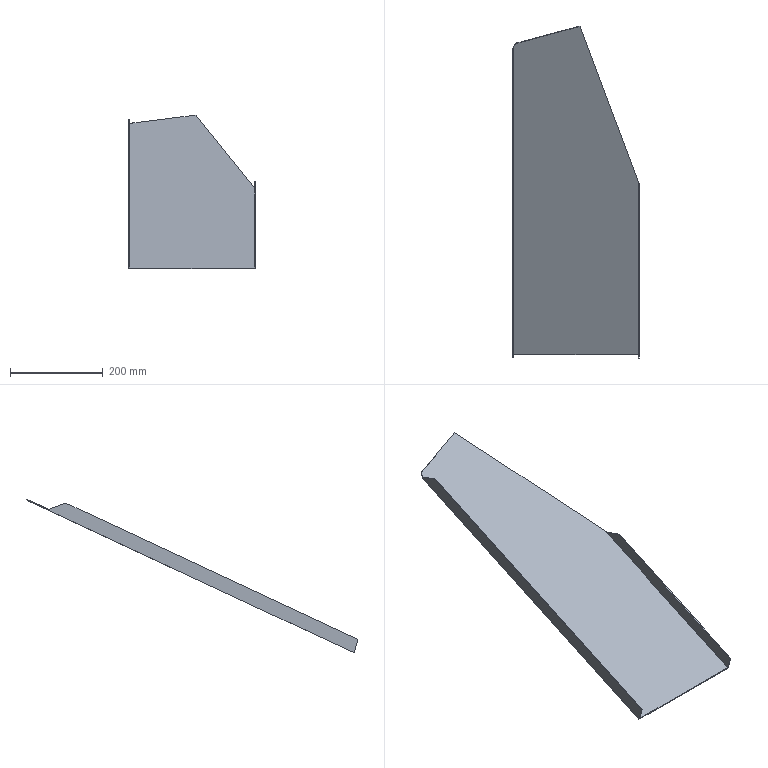Part | NX | features solid 2 | 1 solid | 14 faces | box 271.348 x 713.846 x 331.008 mm | volume 430827 mm3 | plane 13 | spline 1
STEP:
#1=CARTESIAN_POINT('',(380.079,-710.47,-537.234));
#2=VERTEX_POINT('',#1);
#3=CARTESIAN_POINT('',(112.731,-710.47,-537.234));
#4=VERTEX_POINT('',#3);
#5=CARTESIAN_POINT('',(177.1,-710.47,-537.234));
#6=DIRECTION('',(-1.,0.,0.));
#7=VECTOR('',#6,1000.);
#8=LINE('',#5,#7);
#9=EDGE_CURVE('',#2,#4,#8,.T.);
#10=ORIENTED_EDGE('',*,*,#9,.F.);
#11=CARTESIAN_POINT('',(380.079,-342.448,-365.622));
#12=VERTEX_POINT('',#11);
#13=CARTESIAN_POINT('',(380.079,-25.721,-217.93));
#14=DIRECTION('',(0.,0.9063,0.4226));
#15=VECTOR('',#14,1000.);
#16=LINE('',#13,#15);
#17=EDGE_CURVE('',#2,#12,#16,.T.);
#18=ORIENTED_EDGE('',*,*,#17,.T.);
#19=CARTESIAN_POINT('',(382.079,-342.448,-365.622));
#20=VERTEX_POINT('',#19);
#21=CARTESIAN_POINT('',(382.079,-342.448,-365.622));
#22=DIRECTION('',(-1.,0.,0.));
#23=VECTOR('',#22,1000.);
#24=LINE('',#21,#23);
#25=EDGE_CURVE('',#12,#20,#24,.F.);
#26=ORIENTED_EDGE('',*,*,#25,.T.);
#27=CARTESIAN_POINT('',(255.072,-4.828,-208.187));
#28=VERTEX_POINT('',#27);
#29=CARTESIAN_POINT('',(255.072,-4.828,-208.187));
#30=DIRECTION('',(0.3227,-0.8578,-0.4));
#31=VECTOR('',#30,1000.);
#32=LINE('',#29,#31);
#33=EDGE_CURVE('',#28,#20,#32,.T.);
#34=ORIENTED_EDGE('',*,*,#33,.F.);
#35=CARTESIAN_POINT('',(244.53,-7.653,-209.505));
#36=VERTEX_POINT('',#35);
#37=CARTESIAN_POINT('',(255.072,-4.828,-208.187));
#38=CARTESIAN_POINT('',(251.558,-5.77,-208.626));
#39=CARTESIAN_POINT('',(248.044,-6.711,-209.066));
#40=CARTESIAN_POINT('',(244.53,-7.653,-209.505));
#41=B_SPLINE_CURVE_WITH_KNOTS('',3,(#37,#38,#39,#40),.UNSPECIFIED.,.F.,.F.,(4,4),(0.,1.),.PIECEWISE_BEZIER_KNOTS.);
#42=EDGE_CURVE('',#28,#36,#41,.T.);
#43=ORIENTED_EDGE('',*,*,#42,.T.);
#44=CARTESIAN_POINT('',(110.731,-52.513,-230.423));
#45=VERTEX_POINT('',#44);
#46=CARTESIAN_POINT('',(105.417,-66.15,-236.782));
#47=CARTESIAN_POINT('',(107.811,-60.006,-233.917));
#48=CARTESIAN_POINT('',(110.205,-53.862,-231.052));
#49=CARTESIAN_POINT('',(112.599,-47.718,-228.187));
#50=CARTESIAN_POINT('',(112.723,-47.398,-228.038));
#51=CARTESIAN_POINT('',(112.863,-47.087,-227.893));
#52=CARTESIAN_POINT('',(113.169,-46.477,-227.609));
#53=CARTESIAN_POINT('',(113.336,-46.18,-227.47));
#54=CARTESIAN_POINT('',(113.695,-45.599,-227.199));
#55=CARTESIAN_POINT('',(113.888,-45.315,-227.067));
#56=CARTESIAN_POINT('',(114.298,-44.762,-226.809));
#57=CARTESIAN_POINT('',(114.517,-44.493,-226.683));
#58=CARTESIAN_POINT('',(114.865,-44.1,-226.5));
#59=CARTESIAN_POINT('',(114.985,-43.97,-226.44));
#60=CARTESIAN_POINT('',(115.169,-43.779,-226.351));
#61=CARTESIAN_POINT('',(115.232,-43.716,-226.321));
#62=CARTESIAN_POINT('',(115.358,-43.591,-226.263));
#63=CARTESIAN_POINT('',(115.422,-43.53,-226.234));
#64=CARTESIAN_POINT('',(115.745,-43.225,-226.092));
#65=CARTESIAN_POINT('',(116.014,-42.994,-225.984));
#66=CARTESIAN_POINT('',(116.436,-42.666,-225.831));
#67=CARTESIAN_POINT('',(116.579,-42.56,-225.782));
#68=CARTESIAN_POINT('',(116.873,-42.355,-225.686));
#69=CARTESIAN_POINT('',(117.023,-42.256,-225.64));
#70=CARTESIAN_POINT('',(117.33,-42.066,-225.551));
#71=CARTESIAN_POINT('',(117.487,-41.974,-225.509));
#72=CARTESIAN_POINT('',(117.688,-41.865,-225.458));
#73=CARTESIAN_POINT('',(117.729,-41.844,-225.448));
#74=CARTESIAN_POINT('',(117.81,-41.801,-225.428));
#75=CARTESIAN_POINT('',(117.932,-41.739,-225.399));
#76=CARTESIAN_POINT('',(118.055,-41.679,-225.371));
#77=CARTESIAN_POINT('',(118.303,-41.564,-225.318));
#78=CARTESIAN_POINT('',(118.471,-41.493,-225.285));
#79=CARTESIAN_POINT('',(118.809,-41.363,-225.224));
#80=CARTESIAN_POINT('',(118.981,-41.304,-225.196));
#81=CARTESIAN_POINT('',(119.198,-41.238,-225.166));
#82=CARTESIAN_POINT('',(119.263,-41.219,-225.157));
#83=CARTESIAN_POINT('',(119.329,-41.201,-225.148));
#84=CARTESIAN_POINT('',(119.372,-41.189,-225.143));
#85=CARTESIAN_POINT('',(119.394,-41.183,-225.14));
#86=CARTESIAN_POINT('',(119.504,-41.154,-225.126));
#87=CARTESIAN_POINT('',(119.767,-41.083,-225.093));
#88=CARTESIAN_POINT('',(120.733,-40.824,-224.973));
#89=CARTESIAN_POINT('',(123.016,-40.213,-224.687));
#90=CARTESIAN_POINT('',(130.742,-38.142,-223.722));
#91=CARTESIAN_POINT('',(149.005,-33.249,-221.44));
#92=CARTESIAN_POINT('',(188.339,-22.709,-216.526));
#93=CARTESIAN_POINT('',(222.053,-13.676,-212.313));
#94=CARTESIAN_POINT('',(244.53,-7.653,-209.505));
#95=CARTESIAN_POINT('',(251.273,-5.846,-208.662));
#96=CARTESIAN_POINT('',(258.016,-4.039,-207.82));
#97=CARTESIAN_POINT('',(264.759,-2.233,-206.977));
#98=B_SPLINE_CURVE_WITH_KNOTS('',3,(#46,#47,#48,#49,#50,#51,#52,#53,#54,#55,#56,#57,#58,#59,#60,#61,#62,#63,#64,#65,#66,#67,#68,#69,#70,#71,#72,#73,#74,#75,#76,#77,#78,#79,#80,#81,#82,#83,#84,#85,#86,#87,#88,#89,#90,#91,#92,#93,#94,#95,#96,#97),.UNSPECIFIED.,.F.,.F.,(4,3,2,2,2,2,2,2,2,2,2,2,2,2,1,2,2,2,1,2,2,1,1,1,1,1,1,3,4),(-0.15,0.,0.007812,0.01562,0.02344,0.03125,0.03516,0.03711,0.03906,0.04687,0.05078,0.05469,0.05859,0.05957,0.06055,0.0625,0.06641,0.07031,0.07129,0.07178,0.07227,0.07422,0.07812,0.09375,0.125,0.25,0.5,1.,1.15),.UNSPECIFIED.);
#99=EDGE_CURVE('',#45,#36,#98,.T.);
#100=ORIENTED_EDGE('',*,*,#99,.F.);
#101=CARTESIAN_POINT('',(112.731,-52.513,-230.423));
#102=VERTEX_POINT('',#101);
#103=CARTESIAN_POINT('',(110.731,-52.513,-230.423));
#104=DIRECTION('',(-1.,0.,0.));
#105=VECTOR('',#104,1000.);
#106=LINE('',#103,#105);
#107=EDGE_CURVE('',#45,#102,#106,.F.);
#108=ORIENTED_EDGE('',*,*,#107,.T.);
#109=CARTESIAN_POINT('',(112.731,-25.721,-217.93));
#110=DIRECTION('',(0.,-0.9063,-0.4226));
#111=VECTOR('',#110,1000.);
#112=LINE('',#109,#111);
#113=EDGE_CURVE('',#102,#4,#112,.T.);
#114=ORIENTED_EDGE('',*,*,#113,.T.);
#115=EDGE_LOOP('',(#10,#18,#26,#34,#43,#100,#108,#114));
#116=FACE_BOUND('',#115,.T.);
#117=CARTESIAN_POINT('',(177.1,-25.721,-217.93));
#118=DIRECTION('',(0.,-0.4226,0.9063));
#119=DIRECTION('',(0.,-0.9063,-0.4226));
#120=AXIS2_PLACEMENT_3D('',#117,#118,#119);
#121=PLANE('',#120);
#122=ADVANCED_FACE('',(#116),#121,.T.);
#123=CARTESIAN_POINT('',(110.731,-51.668,-232.236));
#124=VERTEX_POINT('',#123);
#125=CARTESIAN_POINT('',(244.53,-6.808,-211.317));
#126=VERTEX_POINT('',#125);
#127=CARTESIAN_POINT('',(105.417,-65.305,-238.595));
#128=CARTESIAN_POINT('',(107.811,-59.161,-235.73));
#129=CARTESIAN_POINT('',(110.205,-53.017,-232.865));
#130=CARTESIAN_POINT('',(112.599,-46.873,-230.));
#131=CARTESIAN_POINT('',(112.723,-46.553,-229.851));
#132=CARTESIAN_POINT('',(112.863,-46.241,-229.705));
#133=CARTESIAN_POINT('',(113.169,-45.632,-229.421));
#134=CARTESIAN_POINT('',(113.336,-45.335,-229.283));
#135=CARTESIAN_POINT('',(113.695,-44.754,-229.012));
#136=CARTESIAN_POINT('',(113.888,-44.47,-228.879));
#137=CARTESIAN_POINT('',(114.298,-43.917,-228.622));
#138=CARTESIAN_POINT('',(114.517,-43.648,-228.496));
#139=CARTESIAN_POINT('',(114.865,-43.254,-228.313));
#140=CARTESIAN_POINT('',(114.985,-43.125,-228.252));
#141=CARTESIAN_POINT('',(115.169,-42.934,-228.163));
#142=CARTESIAN_POINT('',(115.232,-42.871,-228.134));
#143=CARTESIAN_POINT('',(115.358,-42.746,-228.076));
#144=CARTESIAN_POINT('',(115.422,-42.685,-228.047));
#145=CARTESIAN_POINT('',(115.745,-42.38,-227.905));
#146=CARTESIAN_POINT('',(116.014,-42.148,-227.797));
#147=CARTESIAN_POINT('',(116.436,-41.821,-227.644));
#148=CARTESIAN_POINT('',(116.579,-41.715,-227.595));
#149=CARTESIAN_POINT('',(116.873,-41.51,-227.499));
#150=CARTESIAN_POINT('',(117.023,-41.411,-227.453));
#151=CARTESIAN_POINT('',(117.33,-41.22,-227.364));
#152=CARTESIAN_POINT('',(117.487,-41.129,-227.321));
#153=CARTESIAN_POINT('',(117.688,-41.02,-227.271));
#154=CARTESIAN_POINT('',(117.729,-40.999,-227.261));
#155=CARTESIAN_POINT('',(117.81,-40.956,-227.241));
#156=CARTESIAN_POINT('',(117.932,-40.894,-227.212));
#157=CARTESIAN_POINT('',(118.055,-40.834,-227.184));
#158=CARTESIAN_POINT('',(118.303,-40.719,-227.13));
#159=CARTESIAN_POINT('',(118.471,-40.648,-227.097));
#160=CARTESIAN_POINT('',(118.809,-40.518,-227.037));
#161=CARTESIAN_POINT('',(118.981,-40.459,-227.009));
#162=CARTESIAN_POINT('',(119.198,-40.393,-226.978));
#163=CARTESIAN_POINT('',(119.263,-40.374,-226.969));
#164=CARTESIAN_POINT('',(119.329,-40.356,-226.961));
#165=CARTESIAN_POINT('',(119.372,-40.344,-226.955));
#166=CARTESIAN_POINT('',(119.394,-40.338,-226.952));
#167=CARTESIAN_POINT('',(119.504,-40.308,-226.939));
#168=CARTESIAN_POINT('',(119.767,-40.238,-226.906));
#169=CARTESIAN_POINT('',(120.733,-39.979,-226.785));
#170=CARTESIAN_POINT('',(123.016,-39.367,-226.5));
#171=CARTESIAN_POINT('',(130.742,-37.297,-225.535));
#172=CARTESIAN_POINT('',(149.005,-32.404,-223.253));
#173=CARTESIAN_POINT('',(188.339,-21.864,-218.338));
#174=CARTESIAN_POINT('',(222.053,-12.83,-214.126));
#175=CARTESIAN_POINT('',(244.53,-6.808,-211.317));
#176=CARTESIAN_POINT('',(251.273,-5.001,-210.475));
#177=CARTESIAN_POINT('',(258.016,-3.194,-209.632));
#178=CARTESIAN_POINT('',(264.759,-1.387,-208.79));
#179=B_SPLINE_CURVE_WITH_KNOTS('',3,(#127,#128,#129,#130,#131,#132,#133,#134,#135,#136,#137,#138,#139,#140,#141,#142,#143,#144,#145,#146,#147,#148,#149,#150,#151,#152,#153,#154,#155,#156,#157,#158,#159,#160,#161,#162,#163,#164,#165,#166,#167,#168,#169,#170,#171,#172,#173,#174,#175,#176,#177,#178),.UNSPECIFIED.,.F.,.F.,(4,3,2,2,2,2,2,2,2,2,2,2,2,2,1,2,2,2,1,2,2,1,1,1,1,1,1,3,4),(-0.15,0.,0.007812,0.01562,0.02344,0.03125,0.03516,0.03711,0.03906,0.04687,0.05078,0.05469,0.05859,0.05957,0.06055,0.0625,0.06641,0.07031,0.07129,0.07178,0.07227,0.07422,0.07812,0.09375,0.125,0.25,0.5,1.,1.15),.UNSPECIFIED.);
#180=EDGE_CURVE('',#124,#126,#179,.T.);
#181=ORIENTED_EDGE('',*,*,#180,.F.);
#182=CARTESIAN_POINT('',(110.731,-52.091,-231.33));
#183=DIRECTION('',(0.,0.4226,-0.9063));
#184=VECTOR('',#183,1000.);
#185=LINE('',#182,#184);
#186=EDGE_CURVE('',#45,#124,#185,.T.);
#187=ORIENTED_EDGE('',*,*,#186,.F.);
#188=ORIENTED_EDGE('',*,*,#99,.T.);
#189=CARTESIAN_POINT('',(244.53,-7.653,-209.505));
#190=DIRECTION('',(0.,0.4226,-0.9063));
#191=VECTOR('',#190,1000.);
#192=LINE('',#189,#191);
#193=EDGE_CURVE('',#36,#126,#192,.T.);
#194=ORIENTED_EDGE('',*,*,#193,.T.);
#195=EDGE_LOOP('',(#181,#187,#188,#194));
#196=FACE_BOUND('',#195,.T.);
#197=CARTESIAN_POINT('',(110.731,-52.513,-230.423));
#198=CARTESIAN_POINT('',(110.731,-51.668,-232.236));
#199=CARTESIAN_POINT('',(111.249,-51.183,-229.803));
#200=CARTESIAN_POINT('',(111.249,-50.338,-231.616));
#201=CARTESIAN_POINT('',(112.026,-49.189,-228.873));
#202=CARTESIAN_POINT('',(112.026,-48.344,-230.686));
#203=CARTESIAN_POINT('',(113.062,-46.528,-227.632));
#204=CARTESIAN_POINT('',(113.062,-45.682,-229.445));
#205=CARTESIAN_POINT('',(114.237,-44.751,-226.804));
#206=CARTESIAN_POINT('',(114.237,-43.906,-228.616));
#207=CARTESIAN_POINT('',(115.746,-43.133,-226.049));
#208=CARTESIAN_POINT('',(115.746,-42.288,-227.862));
#209=CARTESIAN_POINT('',(117.264,-42.047,-225.543));
#210=CARTESIAN_POINT('',(117.264,-41.202,-227.355));
#211=CARTESIAN_POINT('',(118.643,-41.392,-225.237));
#212=CARTESIAN_POINT('',(118.643,-40.547,-227.05));
#213=CARTESIAN_POINT('',(120.096,-40.991,-225.05));
#214=CARTESIAN_POINT('',(120.096,-40.145,-226.863));
#215=CARTESIAN_POINT('',(122.655,-40.312,-224.734));
#216=CARTESIAN_POINT('',(122.655,-39.467,-226.547));
#217=CARTESIAN_POINT('',(126.302,-39.331,-224.276));
#218=CARTESIAN_POINT('',(126.302,-38.486,-226.089));
#219=CARTESIAN_POINT('',(132.141,-37.768,-223.548));
#220=CARTESIAN_POINT('',(132.141,-36.923,-225.36));
#221=CARTESIAN_POINT('',(139.438,-35.812,-222.635));
#222=CARTESIAN_POINT('',(139.438,-34.967,-224.448));
#223=CARTESIAN_POINT('',(148.196,-33.466,-221.541));
#224=CARTESIAN_POINT('',(148.196,-32.62,-223.354));
#225=CARTESIAN_POINT('',(156.954,-31.119,-220.447));
#226=CARTESIAN_POINT('',(156.954,-30.274,-222.26));
#227=CARTESIAN_POINT('',(165.711,-28.772,-219.353));
#228=CARTESIAN_POINT('',(165.711,-27.927,-221.165));
#229=CARTESIAN_POINT('',(177.388,-25.644,-217.894));
#230=CARTESIAN_POINT('',(177.388,-24.798,-219.706));
#231=CARTESIAN_POINT('',(203.661,-18.604,-214.611));
#232=CARTESIAN_POINT('',(203.661,-17.759,-216.424));
#233=CARTESIAN_POINT('',(227.015,-12.346,-211.693));
#234=CARTESIAN_POINT('',(227.015,-11.501,-213.506));
#235=CARTESIAN_POINT('',(244.53,-7.653,-209.505));
#236=CARTESIAN_POINT('',(244.53,-6.808,-211.317));
#237=B_SPLINE_SURFACE_WITH_KNOTS('',3,1,((#197,#198),(#199,#200),(#201,#202),(#203,#204),(#205,#206),(#207,#208),(#209,#210),(#211,#212),(#213,#214),(#215,#216),(#217,#218),(#219,#220),(#221,#222),(#223,#224),(#225,#226),(#227,#228),(#229,#230),(#231,#232),(#233,#234),(#235,#236)),.UNSPECIFIED.,.F.,.F.,.F.,(4,1,1,1,1,1,1,1,1,1,1,1,1,1,1,1,1,4),(2,2),(-0.03902,-0.006552,0.009682,0.02592,0.04215,0.05839,0.0665,0.07462,0.09086,0.1233,0.1558,0.2207,0.2857,0.3506,0.4156,0.4805,0.6104,1.),(0.,1.),.UNSPECIFIED.);
#238=ADVANCED_FACE('',(#196),#237,.T.);
#239=CARTESIAN_POINT('',(255.072,-3.983,-210.));
#240=VERTEX_POINT('',#239);
#241=CARTESIAN_POINT('',(255.072,-3.983,-210.));
#242=CARTESIAN_POINT('',(251.558,-4.925,-210.439));
#243=CARTESIAN_POINT('',(248.044,-5.866,-210.878));
#244=CARTESIAN_POINT('',(244.53,-6.808,-211.317));
#245=B_SPLINE_CURVE_WITH_KNOTS('',3,(#241,#242,#243,#244),.UNSPECIFIED.,.F.,.F.,(4,4),(0.,1.),.PIECEWISE_BEZIER_KNOTS.);
#246=EDGE_CURVE('',#240,#126,#245,.T.);
#247=ORIENTED_EDGE('',*,*,#246,.T.);
#248=ORIENTED_EDGE('',*,*,#193,.F.);
#249=ORIENTED_EDGE('',*,*,#42,.F.);
#250=CARTESIAN_POINT('',(255.072,-4.828,-208.187));
#251=DIRECTION('',(0.,0.4226,-0.9063));
#252=VECTOR('',#251,1000.);
#253=LINE('',#250,#252);
#254=EDGE_CURVE('',#28,#240,#253,.T.);
#255=ORIENTED_EDGE('',*,*,#254,.T.);
#256=EDGE_LOOP('',(#247,#248,#249,#255));
#257=FACE_BOUND('',#256,.T.);
#258=CARTESIAN_POINT('',(255.072,-4.828,-208.187));
#259=DIRECTION('',(0.2835,-0.8691,-0.4053));
#260=DIRECTION('',(0.,0.4226,-0.9063));
#261=AXIS2_PLACEMENT_3D('',#258,#259,#260);
#262=PLANE('',#261);
#263=ADVANCED_FACE('',(#257),#262,.F.);
#264=CARTESIAN_POINT('',(382.079,-341.602,-367.435));
#265=VERTEX_POINT('',#264);
#266=CARTESIAN_POINT('',(255.072,-3.983,-210.));
#267=DIRECTION('',(0.3227,-0.8578,-0.4));
#268=VECTOR('',#267,1000.);
#269=LINE('',#266,#268);
#270=EDGE_CURVE('',#240,#265,#269,.T.);
#271=ORIENTED_EDGE('',*,*,#270,.F.);
#272=ORIENTED_EDGE('',*,*,#254,.F.);
#273=ORIENTED_EDGE('',*,*,#33,.T.);
#274=CARTESIAN_POINT('',(382.079,-342.448,-365.622));
#275=DIRECTION('',(0.,0.4226,-0.9063));
#276=VECTOR('',#275,1000.);
#277=LINE('',#274,#276);
#278=EDGE_CURVE('',#20,#265,#277,.T.);
#279=ORIENTED_EDGE('',*,*,#278,.T.);
#280=EDGE_LOOP('',(#271,#272,#273,#279));
#281=FACE_BOUND('',#280,.T.);
#282=CARTESIAN_POINT('',(255.072,-4.828,-208.187));
#283=DIRECTION('',(0.9465,0.2925,0.1364));
#284=DIRECTION('',(-0.2952,0.9554,0.));
#285=AXIS2_PLACEMENT_3D('',#282,#283,#284);
#286=PLANE('',#285);
#287=ADVANCED_FACE('',(#281),#286,.T.);
#288=CARTESIAN_POINT('',(382.079,-717.829,-509.77));
#289=VERTEX_POINT('',#288);
#290=CARTESIAN_POINT('',(382.079,-379.658,-352.079));
#291=VERTEX_POINT('',#290);
#292=CARTESIAN_POINT('',(382.079,-852.679,-572.652));
#293=DIRECTION('',(0.,0.9063,0.4226));
#294=VECTOR('',#293,1000.);
#295=LINE('',#292,#294);
#296=EDGE_CURVE('',#289,#291,#295,.T.);
#297=ORIENTED_EDGE('',*,*,#296,.F.);
#298=CARTESIAN_POINT('',(382.079,-709.945,-539.195));
#299=VERTEX_POINT('',#298);
#300=CARTESIAN_POINT('',(382.079,-709.46,-541.004));
#301=DIRECTION('',(0.,0.2588,-0.9659));
#302=VECTOR('',#301,1000.);
#303=LINE('',#300,#302);
#304=EDGE_CURVE('',#289,#299,#303,.T.);
#305=ORIENTED_EDGE('',*,*,#304,.T.);
#306=CARTESIAN_POINT('',(382.079,-730.,-548.547));
#307=DIRECTION('',(0.,0.9063,0.4226));
#308=VECTOR('',#307,1000.);
#309=LINE('',#306,#308);
#310=EDGE_CURVE('',#299,#265,#309,.T.);
#311=ORIENTED_EDGE('',*,*,#310,.T.);
#312=ORIENTED_EDGE('',*,*,#278,.F.);
#313=CARTESIAN_POINT('',(382.079,-706.521,-233.11));
#314=DIRECTION('',(0.,-0.9397,0.342));
#315=VECTOR('',#314,1000.);
#316=LINE('',#313,#315);
#317=EDGE_CURVE('',#20,#291,#316,.T.);
#318=ORIENTED_EDGE('',*,*,#317,.T.);
#319=EDGE_LOOP('',(#297,#305,#311,#312,#318));
#320=FACE_BOUND('',#319,.T.);
#321=CARTESIAN_POINT('',(382.079,-730.845,-546.735));
#322=DIRECTION('',(-1.,0.,0.));
#323=DIRECTION('',(0.,-1.,0.));
#324=AXIS2_PLACEMENT_3D('',#321,#322,#323);
#325=PLANE('',#324);
#326=ADVANCED_FACE('',(#320),#325,.F.);
#327=CARTESIAN_POINT('',(110.731,-709.945,-539.195));
#328=VERTEX_POINT('',#327);
#329=CARTESIAN_POINT('',(110.731,-24.876,-219.742));
#330=DIRECTION('',(0.,0.9063,0.4226));
#331=VECTOR('',#330,1000.);
#332=LINE('',#329,#331);
#333=EDGE_CURVE('',#328,#124,#332,.T.);
#334=ORIENTED_EDGE('',*,*,#333,.F.);
#335=CARTESIAN_POINT('',(110.731,-717.829,-509.77));
#336=VERTEX_POINT('',#335);
#337=CARTESIAN_POINT('',(110.731,-722.22,-493.383));
#338=DIRECTION('',(0.,-0.2588,0.9659));
#339=VECTOR('',#338,1000.);
#340=LINE('',#337,#339);
#341=EDGE_CURVE('',#328,#336,#340,.T.);
#342=ORIENTED_EDGE('',*,*,#341,.T.);
#343=CARTESIAN_POINT('',(110.731,-89.723,-216.88));
#344=VERTEX_POINT('',#343);
#345=CARTESIAN_POINT('',(110.731,-64.347,-205.047));
#346=DIRECTION('',(0.,-0.9063,-0.4226));
#347=VECTOR('',#346,1000.);
#348=LINE('',#345,#347);
#349=EDGE_CURVE('',#344,#336,#348,.T.);
#350=ORIENTED_EDGE('',*,*,#349,.F.);
#351=CARTESIAN_POINT('',(110.731,-51.184,-230.907));
#352=DIRECTION('',(0.,-0.9397,0.342));
#353=VECTOR('',#352,1000.);
#354=LINE('',#351,#353);
#355=EDGE_CURVE('',#344,#45,#354,.F.);
#356=ORIENTED_EDGE('',*,*,#355,.T.);
#357=ORIENTED_EDGE('',*,*,#186,.T.);
#358=EDGE_LOOP('',(#334,#342,#350,#356,#357));
#359=FACE_BOUND('',#358,.T.);
#360=CARTESIAN_POINT('',(110.731,-473.531,-426.747));
#361=DIRECTION('',(1.,0.,0.));
#362=DIRECTION('',(0.,1.,0.));
#363=AXIS2_PLACEMENT_3D('',#360,#361,#362);
#364=PLANE('',#363);
#365=ADVANCED_FACE('',(#359),#364,.F.);
#366=ORIENTED_EDGE('',*,*,#310,.F.);
#367=CARTESIAN_POINT('',(177.1,-709.945,-539.195));
#368=DIRECTION('',(-1.,0.,0.));
#369=VECTOR('',#368,1000.);
#370=LINE('',#367,#369);
#371=EDGE_CURVE('',#299,#328,#370,.T.);
#372=ORIENTED_EDGE('',*,*,#371,.T.);
#373=ORIENTED_EDGE('',*,*,#333,.T.);
#374=ORIENTED_EDGE('',*,*,#180,.T.);
#375=ORIENTED_EDGE('',*,*,#246,.F.);
#376=ORIENTED_EDGE('',*,*,#270,.T.);
#377=EDGE_LOOP('',(#366,#372,#373,#374,#375,#376));
#378=FACE_BOUND('',#377,.T.);
#379=CARTESIAN_POINT('',(177.1,-24.876,-219.742));
#380=DIRECTION('',(0.,-0.4226,0.9063));
#381=DIRECTION('',(0.,-0.9063,-0.4226));
#382=AXIS2_PLACEMENT_3D('',#379,#380,#381);
#383=PLANE('',#382);
#384=ADVANCED_FACE('',(#378),#383,.F.);
#385=CARTESIAN_POINT('',(112.731,-89.723,-216.88));
#386=VERTEX_POINT('',#385);
#387=CARTESIAN_POINT('',(112.731,-717.829,-509.77));
#388=VERTEX_POINT('',#387);
#389=CARTESIAN_POINT('',(112.731,-64.347,-205.047));
#390=DIRECTION('',(0.,-0.9063,-0.4226));
#391=VECTOR('',#390,1000.);
#392=LINE('',#389,#391);
#393=EDGE_CURVE('',#386,#388,#392,.T.);
#394=ORIENTED_EDGE('',*,*,#393,.T.);
#395=CARTESIAN_POINT('',(112.731,-742.588,-417.367));
#396=DIRECTION('',(0.,0.2588,-0.9659));
#397=VECTOR('',#396,1000.);
#398=LINE('',#395,#397);
#399=EDGE_CURVE('',#388,#4,#398,.T.);
#400=ORIENTED_EDGE('',*,*,#399,.T.);
#401=ORIENTED_EDGE('',*,*,#113,.F.);
#402=CARTESIAN_POINT('',(112.731,-52.513,-230.423));
#403=DIRECTION('',(0.,0.9397,-0.342));
#404=VECTOR('',#403,1000.);
#405=LINE('',#402,#404);
#406=EDGE_CURVE('',#102,#386,#405,.F.);
#407=ORIENTED_EDGE('',*,*,#406,.T.);
#408=EDGE_LOOP('',(#394,#400,#401,#407));
#409=FACE_BOUND('',#408,.T.);
#410=CARTESIAN_POINT('',(112.731,-51.668,-232.236));
#411=DIRECTION('',(-1.,0.,0.));
#412=DIRECTION('',(0.,-1.,0.));
#413=AXIS2_PLACEMENT_3D('',#410,#411,#412);
#414=PLANE('',#413);
#415=ADVANCED_FACE('',(#409),#414,.F.);
#416=CARTESIAN_POINT('',(110.731,-717.829,-509.77));
#417=DIRECTION('',(1.,0.,0.));
#418=VECTOR('',#417,1000.);
#419=LINE('',#416,#418);
#420=EDGE_CURVE('',#388,#336,#419,.F.);
#421=ORIENTED_EDGE('',*,*,#420,.F.);
#422=ORIENTED_EDGE('',*,*,#393,.F.);
#423=CARTESIAN_POINT('',(110.731,-89.723,-216.88));
#424=DIRECTION('',(1.,0.,0.));
#425=VECTOR('',#424,1000.);
#426=LINE('',#423,#425);
#427=EDGE_CURVE('',#386,#344,#426,.F.);
#428=ORIENTED_EDGE('',*,*,#427,.T.);
#429=ORIENTED_EDGE('',*,*,#349,.T.);
#430=EDGE_LOOP('',(#421,#422,#428,#429));
#431=FACE_BOUND('',#430,.T.);
#432=CARTESIAN_POINT('',(110.731,-64.347,-205.047));
#433=DIRECTION('',(0.,0.4226,-0.9063));
#434=DIRECTION('',(0.,-0.9063,-0.4226));
#435=AXIS2_PLACEMENT_3D('',#432,#433,#434);
#436=PLANE('',#435);
#437=ADVANCED_FACE('',(#431),#436,.F.);
#438=ORIENTED_EDGE('',*,*,#355,.F.);
#439=ORIENTED_EDGE('',*,*,#427,.F.);
#440=ORIENTED_EDGE('',*,*,#406,.F.);
#441=ORIENTED_EDGE('',*,*,#107,.F.);
#442=EDGE_LOOP('',(#438,#439,#440,#441));
#443=FACE_BOUND('',#442,.T.);
#444=CARTESIAN_POINT('',(110.731,-52.513,-230.423));
#445=DIRECTION('',(0.,-0.342,-0.9397));
#446=DIRECTION('',(0.,0.9397,-0.342));
#447=AXIS2_PLACEMENT_3D('',#444,#445,#446);
#448=PLANE('',#447);
#449=ADVANCED_FACE('',(#443),#448,.F.);
#450=ORIENTED_EDGE('',*,*,#17,.F.);
#451=CARTESIAN_POINT('',(380.079,-717.829,-509.77));
#452=VERTEX_POINT('',#451);
#453=CARTESIAN_POINT('',(380.079,-703.495,-563.265));
#454=DIRECTION('',(0.,-0.2588,0.9659));
#455=VECTOR('',#454,1000.);
#456=LINE('',#453,#455);
#457=EDGE_CURVE('',#2,#452,#456,.T.);
#458=ORIENTED_EDGE('',*,*,#457,.T.);
#459=CARTESIAN_POINT('',(380.079,-379.658,-352.079));
#460=VERTEX_POINT('',#459);
#461=CARTESIAN_POINT('',(380.079,-852.679,-572.652));
#462=DIRECTION('',(0.,0.9063,0.4226));
#463=VECTOR('',#462,1000.);
#464=LINE('',#461,#463);
#465=EDGE_CURVE('',#452,#460,#464,.T.);
#466=ORIENTED_EDGE('',*,*,#465,.T.);
#467=CARTESIAN_POINT('',(380.079,-379.658,-352.079));
#468=DIRECTION('',(0.,0.9397,-0.342));
#469=VECTOR('',#468,1000.);
#470=LINE('',#467,#469);
#471=EDGE_CURVE('',#460,#12,#470,.T.);
#472=ORIENTED_EDGE('',*,*,#471,.T.);
#473=EDGE_LOOP('',(#450,#458,#466,#472));
#474=FACE_BOUND('',#473,.T.);
#475=CARTESIAN_POINT('',(380.079,-840.,-599.841));
#476=DIRECTION('',(1.,0.,0.));
#477=DIRECTION('',(0.,1.,0.));
#478=AXIS2_PLACEMENT_3D('',#475,#476,#477);
#479=PLANE('',#478);
#480=ADVANCED_FACE('',(#474),#479,.F.);
#481=ORIENTED_EDGE('',*,*,#465,.F.);
#482=CARTESIAN_POINT('',(382.079,-717.829,-509.77));
#483=DIRECTION('',(1.,0.,0.));
#484=VECTOR('',#483,1000.);
#485=LINE('',#482,#484);
#486=EDGE_CURVE('',#452,#289,#485,.T.);
#487=ORIENTED_EDGE('',*,*,#486,.T.);
#488=ORIENTED_EDGE('',*,*,#296,.T.);
#489=CARTESIAN_POINT('',(382.079,-379.658,-352.079));
#490=DIRECTION('',(-1.,0.,0.));
#491=VECTOR('',#490,1000.);
#492=LINE('',#489,#491);
#493=EDGE_CURVE('',#291,#460,#492,.T.);
#494=ORIENTED_EDGE('',*,*,#493,.T.);
#495=EDGE_LOOP('',(#481,#487,#488,#494));
#496=FACE_BOUND('',#495,.T.);
#497=CARTESIAN_POINT('',(382.079,-852.679,-572.652));
#498=DIRECTION('',(0.,0.4226,-0.9063));
#499=DIRECTION('',(0.,0.9063,0.4226));
#500=AXIS2_PLACEMENT_3D('',#497,#498,#499);
#501=PLANE('',#500);
#502=ADVANCED_FACE('',(#496),#501,.F.);
#503=ORIENTED_EDGE('',*,*,#317,.F.);
#504=ORIENTED_EDGE('',*,*,#25,.F.);
#505=ORIENTED_EDGE('',*,*,#471,.F.);
#506=ORIENTED_EDGE('',*,*,#493,.F.);
#507=EDGE_LOOP('',(#503,#504,#505,#506));
#508=FACE_BOUND('',#507,.T.);
#509=CARTESIAN_POINT('',(382.079,-379.658,-352.079));
#510=DIRECTION('',(0.,0.342,0.9397));
#511=DIRECTION('',(0.,-0.9397,0.342));
#512=AXIS2_PLACEMENT_3D('',#509,#510,#511);
#513=PLANE('',#512);
#514=ADVANCED_FACE('',(#508),#513,.T.);
#515=ORIENTED_EDGE('',*,*,#399,.F.);
#516=ORIENTED_EDGE('',*,*,#420,.T.);
#517=ORIENTED_EDGE('',*,*,#341,.F.);
#518=ORIENTED_EDGE('',*,*,#371,.F.);
#519=ORIENTED_EDGE('',*,*,#304,.F.);
#520=ORIENTED_EDGE('',*,*,#486,.F.);
#521=ORIENTED_EDGE('',*,*,#457,.F.);
#522=ORIENTED_EDGE('',*,*,#9,.T.);
#523=EDGE_LOOP('',(#515,#516,#517,#518,#519,#520,#521,#522));
#524=FACE_BOUND('',#523,.T.);
#525=CARTESIAN_POINT('',(390.,-706.808,-550.902));
#526=DIRECTION('',(0.,0.9659,0.2588));
#527=DIRECTION('',(0.,-0.2588,0.9659));
#528=AXIS2_PLACEMENT_3D('',#525,#526,#527);
#529=PLANE('',#528);
#530=ADVANCED_FACE('',(#524),#529,.F.);
#531=CLOSED_SHELL('',(#122,#238,#263,#287,#326,#365,#384,#415,#437,#449,#480,#502,#514,#530));
#532=MANIFOLD_SOLID_BREP('',#531);
#533=(LENGTH_UNIT()NAMED_UNIT(*)SI_UNIT(.MILLI.,.METRE.));
#534=UNCERTAINTY_MEASURE_WITH_UNIT(LENGTH_MEASURE(0.0508),#533,'','');
#535=(NAMED_UNIT(*)PLANE_ANGLE_UNIT()SI_UNIT($,.RADIAN.));
#536=(NAMED_UNIT(*)SI_UNIT($,.STERADIAN.)SOLID_ANGLE_UNIT());
#537=(GEOMETRIC_REPRESENTATION_CONTEXT(3)GLOBAL_UNCERTAINTY_ASSIGNED_CONTEXT((#534))GLOBAL_UNIT_ASSIGNED_CONTEXT((#533,#535,#536))REPRESENTATION_CONTEXT('',''));
#538=ADVANCED_BREP_SHAPE_REPRESENTATION('',(#532),#537);